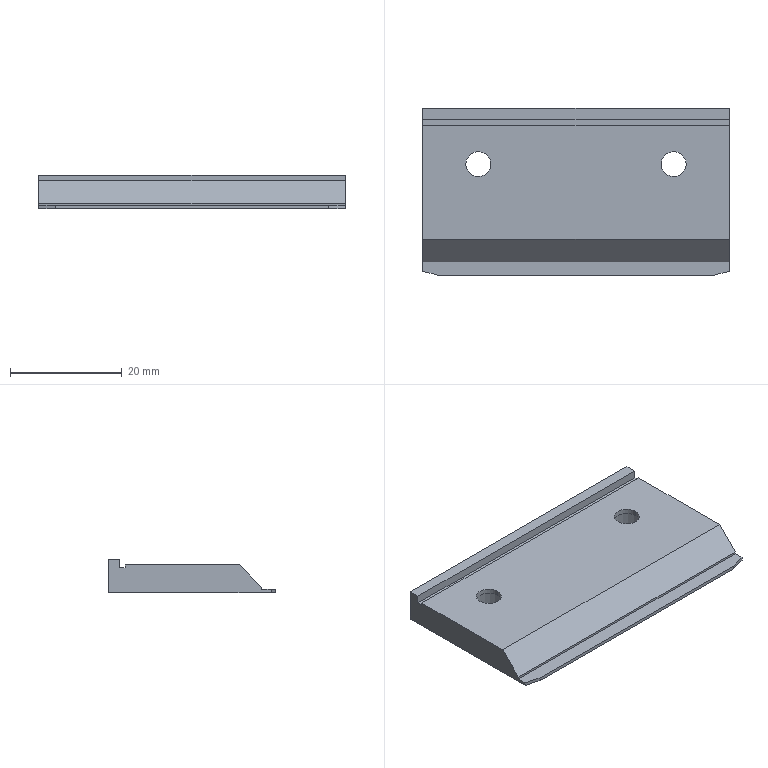Part | STEP file | 11-FG-B03011 | 1 solid | 25 faces | box 55 x 30 x 6 mm | volume 6845 mm3 | plane 17 | cylinder 8 | commonest cylinder face diameters 4.5 x4 8 x4
STEP:
#1=CARTESIAN_POINT('',(14.,20.,-0.9));
#2=VERTEX_POINT('',#1);
#3=CARTESIAN_POINT('',(6.,20.,-0.9));
#4=VERTEX_POINT('',#3);
#5=CARTESIAN_POINT('',(10.,20.,-0.9));
#6=DIRECTION('',(0.,0.,-1.));
#7=DIRECTION('',(-1.,0.,0.));
#8=AXIS2_PLACEMENT_3D('',#5,#6,#7);
#9=CIRCLE('',#8,4.);
#10=EDGE_CURVE('',#2,#4,#9,.T.);
#11=ORIENTED_EDGE('',*,*,#10,.F.);
#12=CARTESIAN_POINT('',(14.,20.,-5.));
#13=VERTEX_POINT('',#12);
#14=CARTESIAN_POINT('',(14.,20.,-5.));
#15=DIRECTION('',(0.,0.,-1.));
#16=VECTOR('',#15,1000.);
#17=LINE('',#14,#16);
#18=EDGE_CURVE('',#2,#13,#17,.T.);
#19=ORIENTED_EDGE('',*,*,#18,.T.);
#20=CARTESIAN_POINT('',(6.,20.,-5.));
#21=VERTEX_POINT('',#20);
#22=CARTESIAN_POINT('',(10.,20.,-5.));
#23=DIRECTION('',(0.,0.,-1.));
#24=DIRECTION('',(-1.,0.,0.));
#25=AXIS2_PLACEMENT_3D('',#22,#23,#24);
#26=CIRCLE('',#25,4.);
#27=EDGE_CURVE('',#13,#21,#26,.T.);
#28=ORIENTED_EDGE('',*,*,#27,.T.);
#29=CARTESIAN_POINT('',(6.,20.,-5.));
#30=DIRECTION('',(0.,0.,-1.));
#31=VECTOR('',#30,1000.);
#32=LINE('',#29,#31);
#33=EDGE_CURVE('',#4,#21,#32,.T.);
#34=ORIENTED_EDGE('',*,*,#33,.F.);
#35=EDGE_LOOP('',(#11,#19,#28,#34));
#36=FACE_OUTER_BOUND('',#35,.T.);
#37=CARTESIAN_POINT('',(10.,20.,-5.));
#38=DIRECTION('',(0.,0.,-1.));
#39=DIRECTION('',(-1.,0.,0.));
#40=AXIS2_PLACEMENT_3D('',#37,#38,#39);
#41=CYLINDRICAL_SURFACE('',#40,4.);
#42=ADVANCED_FACE('',(#36),#41,.F.);
#43=CARTESIAN_POINT('',(12.25,20.,0.));
#44=VERTEX_POINT('',#43);
#45=CARTESIAN_POINT('',(7.75,20.,0.));
#46=VERTEX_POINT('',#45);
#47=CARTESIAN_POINT('',(10.,20.,0.));
#48=DIRECTION('',(0.,0.,-1.));
#49=DIRECTION('',(-1.,0.,0.));
#50=AXIS2_PLACEMENT_3D('',#47,#48,#49);
#51=CIRCLE('',#50,2.25);
#52=EDGE_CURVE('',#44,#46,#51,.T.);
#53=ORIENTED_EDGE('',*,*,#52,.F.);
#54=CARTESIAN_POINT('',(12.25,20.,-0.9));
#55=VERTEX_POINT('',#54);
#56=CARTESIAN_POINT('',(12.25,20.,-5.));
#57=DIRECTION('',(0.,0.,-1.));
#58=VECTOR('',#57,1000.);
#59=LINE('',#56,#58);
#60=EDGE_CURVE('',#44,#55,#59,.T.);
#61=ORIENTED_EDGE('',*,*,#60,.T.);
#62=CARTESIAN_POINT('',(7.75,20.,-0.9));
#63=VERTEX_POINT('',#62);
#64=CARTESIAN_POINT('',(10.,20.,-0.9));
#65=DIRECTION('',(0.,0.,-1.));
#66=DIRECTION('',(-1.,0.,0.));
#67=AXIS2_PLACEMENT_3D('',#64,#65,#66);
#68=CIRCLE('',#67,2.25);
#69=EDGE_CURVE('',#55,#63,#68,.T.);
#70=ORIENTED_EDGE('',*,*,#69,.T.);
#71=CARTESIAN_POINT('',(7.75,20.,-5.));
#72=DIRECTION('',(0.,0.,-1.));
#73=VECTOR('',#72,1000.);
#74=LINE('',#71,#73);
#75=EDGE_CURVE('',#46,#63,#74,.T.);
#76=ORIENTED_EDGE('',*,*,#75,.F.);
#77=EDGE_LOOP('',(#53,#61,#70,#76));
#78=FACE_OUTER_BOUND('',#77,.T.);
#79=CARTESIAN_POINT('',(10.,20.,-5.));
#80=DIRECTION('',(0.,0.,-1.));
#81=DIRECTION('',(-1.,0.,0.));
#82=AXIS2_PLACEMENT_3D('',#79,#80,#81);
#83=CYLINDRICAL_SURFACE('',#82,2.25);
#84=ADVANCED_FACE('',(#78),#83,.F.);
#85=CARTESIAN_POINT('',(49.,20.,-0.9));
#86=VERTEX_POINT('',#85);
#87=CARTESIAN_POINT('',(41.,20.,-0.9));
#88=VERTEX_POINT('',#87);
#89=CARTESIAN_POINT('',(45.,20.,-0.9));
#90=DIRECTION('',(0.,0.,-1.));
#91=DIRECTION('',(-1.,0.,0.));
#92=AXIS2_PLACEMENT_3D('',#89,#90,#91);
#93=CIRCLE('',#92,4.);
#94=EDGE_CURVE('',#86,#88,#93,.T.);
#95=ORIENTED_EDGE('',*,*,#94,.F.);
#96=CARTESIAN_POINT('',(49.,20.,-5.));
#97=VERTEX_POINT('',#96);
#98=CARTESIAN_POINT('',(49.,20.,-5.));
#99=DIRECTION('',(0.,0.,-1.));
#100=VECTOR('',#99,1000.);
#101=LINE('',#98,#100);
#102=EDGE_CURVE('',#86,#97,#101,.T.);
#103=ORIENTED_EDGE('',*,*,#102,.T.);
#104=CARTESIAN_POINT('',(41.,20.,-5.));
#105=VERTEX_POINT('',#104);
#106=CARTESIAN_POINT('',(45.,20.,-5.));
#107=DIRECTION('',(0.,0.,-1.));
#108=DIRECTION('',(-1.,0.,0.));
#109=AXIS2_PLACEMENT_3D('',#106,#107,#108);
#110=CIRCLE('',#109,4.);
#111=EDGE_CURVE('',#97,#105,#110,.T.);
#112=ORIENTED_EDGE('',*,*,#111,.T.);
#113=CARTESIAN_POINT('',(41.,20.,-5.));
#114=DIRECTION('',(0.,0.,-1.));
#115=VECTOR('',#114,1000.);
#116=LINE('',#113,#115);
#117=EDGE_CURVE('',#88,#105,#116,.T.);
#118=ORIENTED_EDGE('',*,*,#117,.F.);
#119=EDGE_LOOP('',(#95,#103,#112,#118));
#120=FACE_OUTER_BOUND('',#119,.T.);
#121=CARTESIAN_POINT('',(45.,20.,-5.));
#122=DIRECTION('',(0.,0.,-1.));
#123=DIRECTION('',(-1.,0.,0.));
#124=AXIS2_PLACEMENT_3D('',#121,#122,#123);
#125=CYLINDRICAL_SURFACE('',#124,4.);
#126=ADVANCED_FACE('',(#120),#125,.F.);
#127=CARTESIAN_POINT('',(47.25,20.,0.));
#128=VERTEX_POINT('',#127);
#129=CARTESIAN_POINT('',(42.75,20.,0.));
#130=VERTEX_POINT('',#129);
#131=CARTESIAN_POINT('',(45.,20.,0.));
#132=DIRECTION('',(0.,0.,-1.));
#133=DIRECTION('',(-1.,0.,0.));
#134=AXIS2_PLACEMENT_3D('',#131,#132,#133);
#135=CIRCLE('',#134,2.25);
#136=EDGE_CURVE('',#128,#130,#135,.T.);
#137=ORIENTED_EDGE('',*,*,#136,.F.);
#138=CARTESIAN_POINT('',(47.25,20.,-0.9));
#139=VERTEX_POINT('',#138);
#140=CARTESIAN_POINT('',(47.25,20.,-5.));
#141=DIRECTION('',(0.,0.,-1.));
#142=VECTOR('',#141,1000.);
#143=LINE('',#140,#142);
#144=EDGE_CURVE('',#128,#139,#143,.T.);
#145=ORIENTED_EDGE('',*,*,#144,.T.);
#146=CARTESIAN_POINT('',(42.75,20.,-0.9));
#147=VERTEX_POINT('',#146);
#148=CARTESIAN_POINT('',(45.,20.,-0.9));
#149=DIRECTION('',(0.,0.,-1.));
#150=DIRECTION('',(-1.,0.,0.));
#151=AXIS2_PLACEMENT_3D('',#148,#149,#150);
#152=CIRCLE('',#151,2.25);
#153=EDGE_CURVE('',#139,#147,#152,.T.);
#154=ORIENTED_EDGE('',*,*,#153,.T.);
#155=CARTESIAN_POINT('',(42.75,20.,-5.));
#156=DIRECTION('',(0.,0.,-1.));
#157=VECTOR('',#156,1000.);
#158=LINE('',#155,#157);
#159=EDGE_CURVE('',#130,#147,#158,.T.);
#160=ORIENTED_EDGE('',*,*,#159,.F.);
#161=EDGE_LOOP('',(#137,#145,#154,#160));
#162=FACE_OUTER_BOUND('',#161,.T.);
#163=CARTESIAN_POINT('',(45.,20.,-5.));
#164=DIRECTION('',(0.,0.,-1.));
#165=DIRECTION('',(-1.,0.,0.));
#166=AXIS2_PLACEMENT_3D('',#163,#164,#165);
#167=CYLINDRICAL_SURFACE('',#166,2.25);
#168=ADVANCED_FACE('',(#162),#167,.F.);
#169=CARTESIAN_POINT('',(10.,20.,0.));
#170=DIRECTION('',(0.,0.,-1.));
#171=DIRECTION('',(-1.,0.,0.));
#172=AXIS2_PLACEMENT_3D('',#169,#170,#171);
#173=CIRCLE('',#172,2.25);
#174=EDGE_CURVE('',#46,#44,#173,.T.);
#175=ORIENTED_EDGE('',*,*,#174,.T.);
#176=ORIENTED_EDGE('',*,*,#52,.T.);
#177=EDGE_LOOP('',(#175,#176));
#178=FACE_BOUND('',#177,.T.);
#179=CARTESIAN_POINT('',(45.,20.,0.));
#180=DIRECTION('',(0.,0.,-1.));
#181=DIRECTION('',(-1.,0.,0.));
#182=AXIS2_PLACEMENT_3D('',#179,#180,#181);
#183=CIRCLE('',#182,2.25);
#184=EDGE_CURVE('',#130,#128,#183,.T.);
#185=ORIENTED_EDGE('',*,*,#184,.T.);
#186=ORIENTED_EDGE('',*,*,#136,.T.);
#187=EDGE_LOOP('',(#185,#186));
#188=FACE_BOUND('',#187,.T.);
#189=CARTESIAN_POINT('',(55.,27.,0.));
#190=VERTEX_POINT('',#189);
#191=CARTESIAN_POINT('',(55.,6.5,0.));
#192=VERTEX_POINT('',#191);
#193=CARTESIAN_POINT('',(55.,30.,0.));
#194=DIRECTION('',(0.,-1.,0.));
#195=VECTOR('',#194,1000.);
#196=LINE('',#193,#195);
#197=EDGE_CURVE('',#190,#192,#196,.T.);
#198=ORIENTED_EDGE('',*,*,#197,.F.);
#199=CARTESIAN_POINT('',(0.,27.,0.));
#200=VERTEX_POINT('',#199);
#201=CARTESIAN_POINT('',(76.,27.,0.));
#202=DIRECTION('',(-1.,0.,0.));
#203=VECTOR('',#202,1000.);
#204=LINE('',#201,#203);
#205=EDGE_CURVE('',#190,#200,#204,.T.);
#206=ORIENTED_EDGE('',*,*,#205,.T.);
#207=CARTESIAN_POINT('',(0.,6.5,0.));
#208=VERTEX_POINT('',#207);
#209=CARTESIAN_POINT('',(0.,30.,0.));
#210=DIRECTION('',(0.,-1.,0.));
#211=VECTOR('',#210,1000.);
#212=LINE('',#209,#211);
#213=EDGE_CURVE('',#200,#208,#212,.T.);
#214=ORIENTED_EDGE('',*,*,#213,.T.);
#215=CARTESIAN_POINT('',(0.,6.5,0.));
#216=DIRECTION('',(1.,0.,0.));
#217=VECTOR('',#216,1000.);
#218=LINE('',#215,#217);
#219=EDGE_CURVE('',#208,#192,#218,.T.);
#220=ORIENTED_EDGE('',*,*,#219,.T.);
#221=EDGE_LOOP('',(#198,#206,#214,#220));
#222=FACE_OUTER_BOUND('',#221,.T.);
#223=CARTESIAN_POINT('',(0.,30.,0.));
#224=DIRECTION('',(0.,0.,-1.));
#225=DIRECTION('',(-1.,0.,0.));
#226=AXIS2_PLACEMENT_3D('',#223,#224,#225);
#227=PLANE('',#226);
#228=ADVANCED_FACE('',(#178,#188,#222),#227,.F.);
#229=ORIENTED_EDGE('',*,*,#213,.F.);
#230=CARTESIAN_POINT('',(0.,27.,-0.5));
#231=VERTEX_POINT('',#230);
#232=CARTESIAN_POINT('',(0.,27.,0.));
#233=DIRECTION('',(0.,0.,1.));
#234=VECTOR('',#233,1000.);
#235=LINE('',#232,#234);
#236=EDGE_CURVE('',#231,#200,#235,.T.);
#237=ORIENTED_EDGE('',*,*,#236,.F.);
#238=CARTESIAN_POINT('',(0.,28.,-0.5));
#239=VERTEX_POINT('',#238);
#240=CARTESIAN_POINT('',(0.,28.,-0.5));
#241=DIRECTION('',(0.,-1.,0.));
#242=VECTOR('',#241,1000.);
#243=LINE('',#240,#242);
#244=EDGE_CURVE('',#239,#231,#243,.T.);
#245=ORIENTED_EDGE('',*,*,#244,.F.);
#246=CARTESIAN_POINT('',(0.,28.,1.));
#247=VERTEX_POINT('',#246);
#248=CARTESIAN_POINT('',(0.,28.,0.));
#249=DIRECTION('',(0.,0.,-1.));
#250=VECTOR('',#249,1000.);
#251=LINE('',#248,#250);
#252=EDGE_CURVE('',#247,#239,#251,.T.);
#253=ORIENTED_EDGE('',*,*,#252,.F.);
#254=CARTESIAN_POINT('',(0.,30.,1.));
#255=VERTEX_POINT('',#254);
#256=CARTESIAN_POINT('',(0.,30.,1.));
#257=DIRECTION('',(0.,-1.,0.));
#258=VECTOR('',#257,1000.);
#259=LINE('',#256,#258);
#260=EDGE_CURVE('',#255,#247,#259,.T.);
#261=ORIENTED_EDGE('',*,*,#260,.F.);
#262=CARTESIAN_POINT('',(0.,30.,-5.));
#263=VERTEX_POINT('',#262);
#264=CARTESIAN_POINT('',(0.,30.,0.));
#265=DIRECTION('',(0.,0.,1.));
#266=VECTOR('',#265,1000.);
#267=LINE('',#264,#266);
#268=EDGE_CURVE('',#263,#255,#267,.T.);
#269=ORIENTED_EDGE('',*,*,#268,.F.);
#270=CARTESIAN_POINT('',(0.,0.8038,-5.));
#271=VERTEX_POINT('',#270);
#272=CARTESIAN_POINT('',(0.,30.,-5.));
#273=DIRECTION('',(0.,-1.,0.));
#274=VECTOR('',#273,1000.);
#275=LINE('',#272,#274);
#276=EDGE_CURVE('',#263,#271,#275,.T.);
#277=ORIENTED_EDGE('',*,*,#276,.T.);
#278=CARTESIAN_POINT('',(0.,0.8038,-4.4));
#279=VERTEX_POINT('',#278);
#280=CARTESIAN_POINT('',(0.,0.8038,0.));
#281=DIRECTION('',(0.,0.,1.));
#282=VECTOR('',#281,1000.);
#283=LINE('',#280,#282);
#284=EDGE_CURVE('',#271,#279,#283,.T.);
#285=ORIENTED_EDGE('',*,*,#284,.T.);
#286=CARTESIAN_POINT('',(0.,2.5,-4.4));
#287=VERTEX_POINT('',#286);
#288=CARTESIAN_POINT('',(0.,0.,-4.4));
#289=DIRECTION('',(0.,1.,0.));
#290=VECTOR('',#289,1000.);
#291=LINE('',#288,#290);
#292=EDGE_CURVE('',#279,#287,#291,.T.);
#293=ORIENTED_EDGE('',*,*,#292,.T.);
#294=CARTESIAN_POINT('',(0.,2.5,-4.));
#295=VERTEX_POINT('',#294);
#296=CARTESIAN_POINT('',(0.,2.5,0.));
#297=DIRECTION('',(0.,0.,1.));
#298=VECTOR('',#297,1000.);
#299=LINE('',#296,#298);
#300=EDGE_CURVE('',#287,#295,#299,.T.);
#301=ORIENTED_EDGE('',*,*,#300,.T.);
#302=CARTESIAN_POINT('',(0.,6.5,0.));
#303=DIRECTION('',(0.,0.7071,0.7071));
#304=VECTOR('',#303,1000.);
#305=LINE('',#302,#304);
#306=EDGE_CURVE('',#295,#208,#305,.T.);
#307=ORIENTED_EDGE('',*,*,#306,.T.);
#308=EDGE_LOOP('',(#229,#237,#245,#253,#261,#269,#277,#285,#293,#301,#307));
#309=FACE_OUTER_BOUND('',#308,.T.);
#310=CARTESIAN_POINT('',(0.,30.,0.));
#311=DIRECTION('',(1.,0.,0.));
#312=DIRECTION('',(0.,0.,-1.));
#313=AXIS2_PLACEMENT_3D('',#310,#311,#312);
#314=PLANE('',#313);
#315=ADVANCED_FACE('',(#309),#314,.F.);
#316=CARTESIAN_POINT('',(55.,28.,-0.5));
#317=VERTEX_POINT('',#316);
#318=CARTESIAN_POINT('',(55.,27.,-0.5));
#319=VERTEX_POINT('',#318);
#320=CARTESIAN_POINT('',(55.,30.,-0.5));
#321=DIRECTION('',(0.,-1.,0.));
#322=VECTOR('',#321,1000.);
#323=LINE('',#320,#322);
#324=EDGE_CURVE('',#317,#319,#323,.T.);
#325=ORIENTED_EDGE('',*,*,#324,.T.);
#326=CARTESIAN_POINT('',(55.,27.,0.));
#327=DIRECTION('',(0.,0.,1.));
#328=VECTOR('',#327,1000.);
#329=LINE('',#326,#328);
#330=EDGE_CURVE('',#319,#190,#329,.T.);
#331=ORIENTED_EDGE('',*,*,#330,.T.);
#332=ORIENTED_EDGE('',*,*,#197,.T.);
#333=CARTESIAN_POINT('',(55.,2.5,-4.));
#334=VERTEX_POINT('',#333);
#335=CARTESIAN_POINT('',(55.,6.5,0.));
#336=DIRECTION('',(0.,-0.7071,-0.7071));
#337=VECTOR('',#336,1000.);
#338=LINE('',#335,#337);
#339=EDGE_CURVE('',#192,#334,#338,.T.);
#340=ORIENTED_EDGE('',*,*,#339,.T.);
#341=CARTESIAN_POINT('',(55.,2.5,-4.4));
#342=VERTEX_POINT('',#341);
#343=CARTESIAN_POINT('',(55.,2.5,0.));
#344=DIRECTION('',(0.,0.,1.));
#345=VECTOR('',#344,1000.);
#346=LINE('',#343,#345);
#347=EDGE_CURVE('',#342,#334,#346,.T.);
#348=ORIENTED_EDGE('',*,*,#347,.F.);
#349=CARTESIAN_POINT('',(55.,0.8038,-4.4));
#350=VERTEX_POINT('',#349);
#351=CARTESIAN_POINT('',(55.,0.,-4.4));
#352=DIRECTION('',(0.,1.,0.));
#353=VECTOR('',#352,1000.);
#354=LINE('',#351,#353);
#355=EDGE_CURVE('',#350,#342,#354,.T.);
#356=ORIENTED_EDGE('',*,*,#355,.F.);
#357=CARTESIAN_POINT('',(55.,0.8038,-5.));
#358=VERTEX_POINT('',#357);
#359=CARTESIAN_POINT('',(55.,0.8038,-5.));
#360=DIRECTION('',(0.,0.,-1.));
#361=VECTOR('',#360,1000.);
#362=LINE('',#359,#361);
#363=EDGE_CURVE('',#350,#358,#362,.T.);
#364=ORIENTED_EDGE('',*,*,#363,.T.);
#365=CARTESIAN_POINT('',(55.,30.,-5.));
#366=VERTEX_POINT('',#365);
#367=CARTESIAN_POINT('',(55.,30.,-5.));
#368=DIRECTION('',(0.,-1.,0.));
#369=VECTOR('',#368,1000.);
#370=LINE('',#367,#369);
#371=EDGE_CURVE('',#366,#358,#370,.T.);
#372=ORIENTED_EDGE('',*,*,#371,.F.);
#373=CARTESIAN_POINT('',(55.,30.,1.));
#374=VERTEX_POINT('',#373);
#375=CARTESIAN_POINT('',(55.,30.,0.));
#376=DIRECTION('',(0.,0.,-1.));
#377=VECTOR('',#376,1000.);
#378=LINE('',#375,#377);
#379=EDGE_CURVE('',#374,#366,#378,.T.);
#380=ORIENTED_EDGE('',*,*,#379,.F.);
#381=CARTESIAN_POINT('',(55.,28.,1.));
#382=VERTEX_POINT('',#381);
#383=CARTESIAN_POINT('',(55.,30.,1.));
#384=DIRECTION('',(0.,-1.,0.));
#385=VECTOR('',#384,1000.);
#386=LINE('',#383,#385);
#387=EDGE_CURVE('',#374,#382,#386,.T.);
#388=ORIENTED_EDGE('',*,*,#387,.T.);
#389=CARTESIAN_POINT('',(55.,28.,0.));
#390=DIRECTION('',(0.,0.,-1.));
#391=VECTOR('',#390,1000.);
#392=LINE('',#389,#391);
#393=EDGE_CURVE('',#382,#317,#392,.T.);
#394=ORIENTED_EDGE('',*,*,#393,.T.);
#395=EDGE_LOOP('',(#325,#331,#332,#340,#348,#356,#364,#372,#380,#388,#394));
#396=FACE_OUTER_BOUND('',#395,.T.);
#397=CARTESIAN_POINT('',(55.,30.,0.));
#398=DIRECTION('',(-1.,0.,0.));
#399=DIRECTION('',(0.,0.,1.));
#400=AXIS2_PLACEMENT_3D('',#397,#398,#399);
#401=PLANE('',#400);
#402=ADVANCED_FACE('',(#396),#401,.F.);
#403=CARTESIAN_POINT('',(10.,20.,-5.));
#404=DIRECTION('',(0.,0.,-1.));
#405=DIRECTION('',(-1.,0.,0.));
#406=AXIS2_PLACEMENT_3D('',#403,#404,#405);
#407=CIRCLE('',#406,4.);
#408=EDGE_CURVE('',#21,#13,#407,.T.);
#409=ORIENTED_EDGE('',*,*,#408,.F.);
#410=ORIENTED_EDGE('',*,*,#27,.F.);
#411=EDGE_LOOP('',(#409,#410));
#412=FACE_BOUND('',#411,.T.);
#413=CARTESIAN_POINT('',(45.,20.,-5.));
#414=DIRECTION('',(0.,0.,-1.));
#415=DIRECTION('',(-1.,0.,0.));
#416=AXIS2_PLACEMENT_3D('',#413,#414,#415);
#417=CIRCLE('',#416,4.);
#418=EDGE_CURVE('',#105,#97,#417,.T.);
#419=ORIENTED_EDGE('',*,*,#418,.F.);
#420=ORIENTED_EDGE('',*,*,#111,.F.);
#421=EDGE_LOOP('',(#419,#420));
#422=FACE_BOUND('',#421,.T.);
#423=ORIENTED_EDGE('',*,*,#371,.T.);
#424=CARTESIAN_POINT('',(52.,0.,-5.));
#425=VERTEX_POINT('',#424);
#426=CARTESIAN_POINT('',(55.,0.8038,-5.));
#427=DIRECTION('',(-0.9659,-0.2588,0.));
#428=VECTOR('',#427,1000.);
#429=LINE('',#426,#428);
#430=EDGE_CURVE('',#358,#425,#429,.T.);
#431=ORIENTED_EDGE('',*,*,#430,.T.);
#432=CARTESIAN_POINT('',(3.,0.,-5.));
#433=VERTEX_POINT('',#432);
#434=CARTESIAN_POINT('',(0.,0.,-5.));
#435=DIRECTION('',(-1.,0.,0.));
#436=VECTOR('',#435,1000.);
#437=LINE('',#434,#436);
#438=EDGE_CURVE('',#425,#433,#437,.T.);
#439=ORIENTED_EDGE('',*,*,#438,.T.);
#440=CARTESIAN_POINT('',(0.,0.8038,-5.));
#441=DIRECTION('',(-0.9659,0.2588,0.));
#442=VECTOR('',#441,1000.);
#443=LINE('',#440,#442);
#444=EDGE_CURVE('',#433,#271,#443,.T.);
#445=ORIENTED_EDGE('',*,*,#444,.T.);
#446=ORIENTED_EDGE('',*,*,#276,.F.);
#447=CARTESIAN_POINT('',(0.,30.,-5.));
#448=DIRECTION('',(-1.,0.,0.));
#449=VECTOR('',#448,1000.);
#450=LINE('',#447,#449);
#451=EDGE_CURVE('',#366,#263,#450,.T.);
#452=ORIENTED_EDGE('',*,*,#451,.F.);
#453=EDGE_LOOP('',(#423,#431,#439,#445,#446,#452));
#454=FACE_OUTER_BOUND('',#453,.T.);
#455=CARTESIAN_POINT('',(0.,30.,-5.));
#456=DIRECTION('',(0.,0.,1.));
#457=DIRECTION('',(1.,0.,0.));
#458=AXIS2_PLACEMENT_3D('',#455,#456,#457);
#459=PLANE('',#458);
#460=ADVANCED_FACE('',(#412,#422,#454),#459,.F.);
#461=ORIENTED_EDGE('',*,*,#268,.T.);
#462=CARTESIAN_POINT('',(0.,30.,1.));
#463=DIRECTION('',(1.,0.,0.));
#464=VECTOR('',#463,1000.);
#465=LINE('',#462,#464);
#466=EDGE_CURVE('',#255,#374,#465,.T.);
#467=ORIENTED_EDGE('',*,*,#466,.T.);
#468=ORIENTED_EDGE('',*,*,#379,.T.);
#469=ORIENTED_EDGE('',*,*,#451,.T.);
#470=EDGE_LOOP('',(#461,#467,#468,#469));
#471=FACE_OUTER_BOUND('',#470,.T.);
#472=CARTESIAN_POINT('',(0.,30.,-5.));
#473=DIRECTION('',(0.,-1.,0.));
#474=DIRECTION('',(0.,0.,-1.));
#475=AXIS2_PLACEMENT_3D('',#472,#473,#474);
#476=PLANE('',#475);
#477=ADVANCED_FACE('',(#471),#476,.F.);
#478=CARTESIAN_POINT('',(3.,0.,-4.4));
#479=VERTEX_POINT('',#478);
#480=CARTESIAN_POINT('',(52.,0.,-4.4));
#481=VERTEX_POINT('',#480);
#482=CARTESIAN_POINT('',(0.,0.,-4.4));
#483=DIRECTION('',(1.,0.,0.));
#484=VECTOR('',#483,1000.);
#485=LINE('',#482,#484);
#486=EDGE_CURVE('',#479,#481,#485,.T.);
#487=ORIENTED_EDGE('',*,*,#486,.F.);
#488=CARTESIAN_POINT('',(3.,0.,-5.));
#489=DIRECTION('',(0.,0.,-1.));
#490=VECTOR('',#489,1000.);
#491=LINE('',#488,#490);
#492=EDGE_CURVE('',#479,#433,#491,.T.);
#493=ORIENTED_EDGE('',*,*,#492,.T.);
#494=ORIENTED_EDGE('',*,*,#438,.F.);
#495=CARTESIAN_POINT('',(52.,0.,0.));
#496=DIRECTION('',(0.,0.,1.));
#497=VECTOR('',#496,1000.);
#498=LINE('',#495,#497);
#499=EDGE_CURVE('',#425,#481,#498,.T.);
#500=ORIENTED_EDGE('',*,*,#499,.T.);
#501=EDGE_LOOP('',(#487,#493,#494,#500));
#502=FACE_OUTER_BOUND('',#501,.T.);
#503=CARTESIAN_POINT('',(0.,0.,-5.));
#504=DIRECTION('',(0.,-1.,0.));
#505=DIRECTION('',(0.,0.,-1.));
#506=AXIS2_PLACEMENT_3D('',#503,#504,#505);
#507=PLANE('',#506);
#508=ADVANCED_FACE('',(#502),#507,.T.);
#509=CARTESIAN_POINT('',(55.,0.8038,-4.4));
#510=DIRECTION('',(0.9659,0.2588,0.));
#511=VECTOR('',#510,1000.);
#512=LINE('',#509,#511);
#513=EDGE_CURVE('',#481,#350,#512,.T.);
#514=ORIENTED_EDGE('',*,*,#513,.F.);
#515=ORIENTED_EDGE('',*,*,#499,.F.);
#516=ORIENTED_EDGE('',*,*,#430,.F.);
#517=ORIENTED_EDGE('',*,*,#363,.F.);
#518=EDGE_LOOP('',(#514,#515,#516,#517));
#519=FACE_OUTER_BOUND('',#518,.T.);
#520=CARTESIAN_POINT('',(55.,0.8038,0.));
#521=DIRECTION('',(0.2588,-0.9659,0.));
#522=DIRECTION('',(0.9659,0.2588,0.));
#523=AXIS2_PLACEMENT_3D('',#520,#521,#522);
#524=PLANE('',#523);
#525=ADVANCED_FACE('',(#519),#524,.T.);
#526=CARTESIAN_POINT('',(0.,0.8038,-4.4));
#527=DIRECTION('',(0.9659,-0.2588,0.));
#528=VECTOR('',#527,1000.);
#529=LINE('',#526,#528);
#530=EDGE_CURVE('',#279,#479,#529,.T.);
#531=ORIENTED_EDGE('',*,*,#530,.F.);
#532=ORIENTED_EDGE('',*,*,#284,.F.);
#533=ORIENTED_EDGE('',*,*,#444,.F.);
#534=ORIENTED_EDGE('',*,*,#492,.F.);
#535=EDGE_LOOP('',(#531,#532,#533,#534));
#536=FACE_OUTER_BOUND('',#535,.T.);
#537=CARTESIAN_POINT('',(0.,0.8038,0.));
#538=DIRECTION('',(-0.2588,-0.9659,0.));
#539=DIRECTION('',(0.9659,-0.2588,0.));
#540=AXIS2_PLACEMENT_3D('',#537,#538,#539);
#541=PLANE('',#540);
#542=ADVANCED_FACE('',(#536),#541,.T.);
#543=ORIENTED_EDGE('',*,*,#347,.T.);
#544=CARTESIAN_POINT('',(0.,2.5,-4.));
#545=DIRECTION('',(-1.,0.,0.));
#546=VECTOR('',#545,1000.);
#547=LINE('',#544,#546);
#548=EDGE_CURVE('',#334,#295,#547,.T.);
#549=ORIENTED_EDGE('',*,*,#548,.T.);
#550=ORIENTED_EDGE('',*,*,#300,.F.);
#551=CARTESIAN_POINT('',(0.,2.5,-4.4));
#552=DIRECTION('',(1.,0.,0.));
#553=VECTOR('',#552,1000.);
#554=LINE('',#551,#553);
#555=EDGE_CURVE('',#287,#342,#554,.T.);
#556=ORIENTED_EDGE('',*,*,#555,.T.);
#557=EDGE_LOOP('',(#543,#549,#550,#556));
#558=FACE_OUTER_BOUND('',#557,.T.);
#559=CARTESIAN_POINT('',(0.,2.5,0.));
#560=DIRECTION('',(0.,1.,0.));
#561=DIRECTION('',(0.,0.,1.));
#562=AXIS2_PLACEMENT_3D('',#559,#560,#561);
#563=PLANE('',#562);
#564=ADVANCED_FACE('',(#558),#563,.F.);
#565=ORIENTED_EDGE('',*,*,#513,.T.);
#566=ORIENTED_EDGE('',*,*,#355,.T.);
#567=ORIENTED_EDGE('',*,*,#555,.F.);
#568=ORIENTED_EDGE('',*,*,#292,.F.);
#569=ORIENTED_EDGE('',*,*,#530,.T.);
#570=ORIENTED_EDGE('',*,*,#486,.T.);
#571=EDGE_LOOP('',(#565,#566,#567,#568,#569,#570));
#572=FACE_OUTER_BOUND('',#571,.T.);
#573=CARTESIAN_POINT('',(0.,0.,-4.4));
#574=DIRECTION('',(0.,0.,-1.));
#575=DIRECTION('',(-1.,0.,0.));
#576=AXIS2_PLACEMENT_3D('',#573,#574,#575);
#577=PLANE('',#576);
#578=ADVANCED_FACE('',(#572),#577,.F.);
#579=ORIENTED_EDGE('',*,*,#306,.F.);
#580=ORIENTED_EDGE('',*,*,#548,.F.);
#581=ORIENTED_EDGE('',*,*,#339,.F.);
#582=ORIENTED_EDGE('',*,*,#219,.F.);
#583=EDGE_LOOP('',(#579,#580,#581,#582));
#584=FACE_OUTER_BOUND('',#583,.T.);
#585=CARTESIAN_POINT('',(0.,6.5,0.));
#586=DIRECTION('',(0.,0.7071,-0.7071));
#587=DIRECTION('',(0.,0.7071,0.7071));
#588=AXIS2_PLACEMENT_3D('',#585,#586,#587);
#589=PLANE('',#588);
#590=ADVANCED_FACE('',(#584),#589,.F.);
#591=ORIENTED_EDGE('',*,*,#393,.F.);
#592=CARTESIAN_POINT('',(0.,28.,1.));
#593=DIRECTION('',(1.,0.,0.));
#594=VECTOR('',#593,1000.);
#595=LINE('',#592,#594);
#596=EDGE_CURVE('',#247,#382,#595,.T.);
#597=ORIENTED_EDGE('',*,*,#596,.F.);
#598=ORIENTED_EDGE('',*,*,#252,.T.);
#599=CARTESIAN_POINT('',(76.,28.,-0.5));
#600=DIRECTION('',(-1.,0.,0.));
#601=VECTOR('',#600,1000.);
#602=LINE('',#599,#601);
#603=EDGE_CURVE('',#317,#239,#602,.T.);
#604=ORIENTED_EDGE('',*,*,#603,.F.);
#605=EDGE_LOOP('',(#591,#597,#598,#604));
#606=FACE_OUTER_BOUND('',#605,.T.);
#607=CARTESIAN_POINT('',(0.,28.,0.));
#608=DIRECTION('',(0.,-1.,0.));
#609=DIRECTION('',(0.,0.,-1.));
#610=AXIS2_PLACEMENT_3D('',#607,#608,#609);
#611=PLANE('',#610);
#612=ADVANCED_FACE('',(#606),#611,.T.);
#613=ORIENTED_EDGE('',*,*,#387,.F.);
#614=ORIENTED_EDGE('',*,*,#466,.F.);
#615=ORIENTED_EDGE('',*,*,#260,.T.);
#616=ORIENTED_EDGE('',*,*,#596,.T.);
#617=EDGE_LOOP('',(#613,#614,#615,#616));
#618=FACE_OUTER_BOUND('',#617,.T.);
#619=CARTESIAN_POINT('',(0.,30.,1.));
#620=DIRECTION('',(0.,0.,1.));
#621=DIRECTION('',(1.,0.,0.));
#622=AXIS2_PLACEMENT_3D('',#619,#620,#621);
#623=PLANE('',#622);
#624=ADVANCED_FACE('',(#618),#623,.T.);
#625=ORIENTED_EDGE('',*,*,#144,.F.);
#626=ORIENTED_EDGE('',*,*,#184,.F.);
#627=ORIENTED_EDGE('',*,*,#159,.T.);
#628=CARTESIAN_POINT('',(45.,20.,-0.9));
#629=DIRECTION('',(0.,0.,-1.));
#630=DIRECTION('',(-1.,0.,0.));
#631=AXIS2_PLACEMENT_3D('',#628,#629,#630);
#632=CIRCLE('',#631,2.25);
#633=EDGE_CURVE('',#147,#139,#632,.T.);
#634=ORIENTED_EDGE('',*,*,#633,.T.);
#635=EDGE_LOOP('',(#625,#626,#627,#634));
#636=FACE_OUTER_BOUND('',#635,.T.);
#637=CARTESIAN_POINT('',(45.,20.,-5.));
#638=DIRECTION('',(0.,0.,-1.));
#639=DIRECTION('',(-1.,0.,0.));
#640=AXIS2_PLACEMENT_3D('',#637,#638,#639);
#641=CYLINDRICAL_SURFACE('',#640,2.25);
#642=ADVANCED_FACE('',(#636),#641,.F.);
#643=ORIENTED_EDGE('',*,*,#102,.F.);
#644=CARTESIAN_POINT('',(45.,20.,-0.9));
#645=DIRECTION('',(0.,0.,-1.));
#646=DIRECTION('',(-1.,0.,0.));
#647=AXIS2_PLACEMENT_3D('',#644,#645,#646);
#648=CIRCLE('',#647,4.);
#649=EDGE_CURVE('',#88,#86,#648,.T.);
#650=ORIENTED_EDGE('',*,*,#649,.F.);
#651=ORIENTED_EDGE('',*,*,#117,.T.);
#652=ORIENTED_EDGE('',*,*,#418,.T.);
#653=EDGE_LOOP('',(#643,#650,#651,#652));
#654=FACE_OUTER_BOUND('',#653,.T.);
#655=CARTESIAN_POINT('',(45.,20.,-5.));
#656=DIRECTION('',(0.,0.,-1.));
#657=DIRECTION('',(-1.,0.,0.));
#658=AXIS2_PLACEMENT_3D('',#655,#656,#657);
#659=CYLINDRICAL_SURFACE('',#658,4.);
#660=ADVANCED_FACE('',(#654),#659,.F.);
#661=ORIENTED_EDGE('',*,*,#60,.F.);
#662=ORIENTED_EDGE('',*,*,#174,.F.);
#663=ORIENTED_EDGE('',*,*,#75,.T.);
#664=CARTESIAN_POINT('',(10.,20.,-0.9));
#665=DIRECTION('',(0.,0.,-1.));
#666=DIRECTION('',(-1.,0.,0.));
#667=AXIS2_PLACEMENT_3D('',#664,#665,#666);
#668=CIRCLE('',#667,2.25);
#669=EDGE_CURVE('',#63,#55,#668,.T.);
#670=ORIENTED_EDGE('',*,*,#669,.T.);
#671=EDGE_LOOP('',(#661,#662,#663,#670));
#672=FACE_OUTER_BOUND('',#671,.T.);
#673=CARTESIAN_POINT('',(10.,20.,-5.));
#674=DIRECTION('',(0.,0.,-1.));
#675=DIRECTION('',(-1.,0.,0.));
#676=AXIS2_PLACEMENT_3D('',#673,#674,#675);
#677=CYLINDRICAL_SURFACE('',#676,2.25);
#678=ADVANCED_FACE('',(#672),#677,.F.);
#679=ORIENTED_EDGE('',*,*,#18,.F.);
#680=CARTESIAN_POINT('',(10.,20.,-0.9));
#681=DIRECTION('',(0.,0.,-1.));
#682=DIRECTION('',(-1.,0.,0.));
#683=AXIS2_PLACEMENT_3D('',#680,#681,#682);
#684=CIRCLE('',#683,4.);
#685=EDGE_CURVE('',#4,#2,#684,.T.);
#686=ORIENTED_EDGE('',*,*,#685,.F.);
#687=ORIENTED_EDGE('',*,*,#33,.T.);
#688=ORIENTED_EDGE('',*,*,#408,.T.);
#689=EDGE_LOOP('',(#679,#686,#687,#688));
#690=FACE_OUTER_BOUND('',#689,.T.);
#691=CARTESIAN_POINT('',(10.,20.,-5.));
#692=DIRECTION('',(0.,0.,-1.));
#693=DIRECTION('',(-1.,0.,0.));
#694=AXIS2_PLACEMENT_3D('',#691,#692,#693);
#695=CYLINDRICAL_SURFACE('',#694,4.);
#696=ADVANCED_FACE('',(#690),#695,.F.);
#697=ORIENTED_EDGE('',*,*,#649,.T.);
#698=ORIENTED_EDGE('',*,*,#94,.T.);
#699=EDGE_LOOP('',(#697,#698));
#700=FACE_OUTER_BOUND('',#699,.T.);
#701=ORIENTED_EDGE('',*,*,#633,.F.);
#702=ORIENTED_EDGE('',*,*,#153,.F.);
#703=EDGE_LOOP('',(#701,#702));
#704=FACE_BOUND('',#703,.T.);
#705=CARTESIAN_POINT('',(45.,20.,-0.9));
#706=DIRECTION('',(0.,0.,-1.));
#707=DIRECTION('',(-1.,0.,0.));
#708=AXIS2_PLACEMENT_3D('',#705,#706,#707);
#709=PLANE('',#708);
#710=ADVANCED_FACE('',(#700,#704),#709,.T.);
#711=ORIENTED_EDGE('',*,*,#685,.T.);
#712=ORIENTED_EDGE('',*,*,#10,.T.);
#713=EDGE_LOOP('',(#711,#712));
#714=FACE_OUTER_BOUND('',#713,.T.);
#715=ORIENTED_EDGE('',*,*,#669,.F.);
#716=ORIENTED_EDGE('',*,*,#69,.F.);
#717=EDGE_LOOP('',(#715,#716));
#718=FACE_BOUND('',#717,.T.);
#719=CARTESIAN_POINT('',(10.,20.,-0.9));
#720=DIRECTION('',(0.,0.,-1.));
#721=DIRECTION('',(-1.,0.,0.));
#722=AXIS2_PLACEMENT_3D('',#719,#720,#721);
#723=PLANE('',#722);
#724=ADVANCED_FACE('',(#714,#718),#723,.T.);
#725=CARTESIAN_POINT('',(76.,27.,-0.5));
#726=DIRECTION('',(-1.,0.,0.));
#727=VECTOR('',#726,1000.);
#728=LINE('',#725,#727);
#729=EDGE_CURVE('',#319,#231,#728,.T.);
#730=ORIENTED_EDGE('',*,*,#729,.T.);
#731=ORIENTED_EDGE('',*,*,#236,.T.);
#732=ORIENTED_EDGE('',*,*,#205,.F.);
#733=ORIENTED_EDGE('',*,*,#330,.F.);
#734=EDGE_LOOP('',(#730,#731,#732,#733));
#735=FACE_OUTER_BOUND('',#734,.T.);
#736=CARTESIAN_POINT('',(76.,27.,0.));
#737=DIRECTION('',(0.,-1.,0.));
#738=DIRECTION('',(0.,0.,-1.));
#739=AXIS2_PLACEMENT_3D('',#736,#737,#738);
#740=PLANE('',#739);
#741=ADVANCED_FACE('',(#735),#740,.F.);
#742=ORIENTED_EDGE('',*,*,#603,.T.);
#743=ORIENTED_EDGE('',*,*,#244,.T.);
#744=ORIENTED_EDGE('',*,*,#729,.F.);
#745=ORIENTED_EDGE('',*,*,#324,.F.);
#746=EDGE_LOOP('',(#742,#743,#744,#745));
#747=FACE_OUTER_BOUND('',#746,.T.);
#748=CARTESIAN_POINT('',(76.,28.,-0.5));
#749=DIRECTION('',(0.,0.,-1.));
#750=DIRECTION('',(-1.,0.,0.));
#751=AXIS2_PLACEMENT_3D('',#748,#749,#750);
#752=PLANE('',#751);
#753=ADVANCED_FACE('',(#747),#752,.F.);
#754=CLOSED_SHELL('',(#42,#84,#126,#168,#228,#315,#402,#460,#477,#508,#525,#542,#564,#578,#590,#612,#624,#642,#660,#678,#696,#710,#724,#741,#753));
#755=MANIFOLD_SOLID_BREP('',#754);
#756=CARTESIAN_POINT('',(0.,0.,0.));
#757=DIRECTION('',(0.,0.,1.));
#758=DIRECTION('',(1.,0.,0.));
#759=AXIS2_PLACEMENT_3D('',#756,#757,#758);
#760=(LENGTH_UNIT()NAMED_UNIT(*)SI_UNIT(.MILLI.,.METRE.));
#761=UNCERTAINTY_MEASURE_WITH_UNIT(LENGTH_MEASURE(0.00001),#760,'','');
#762=(NAMED_UNIT(*)PLANE_ANGLE_UNIT()SI_UNIT($,.RADIAN.));
#763=(NAMED_UNIT(*)SI_UNIT($,.STERADIAN.)SOLID_ANGLE_UNIT());
#764=(GEOMETRIC_REPRESENTATION_CONTEXT(3)GLOBAL_UNCERTAINTY_ASSIGNED_CONTEXT((#761))GLOBAL_UNIT_ASSIGNED_CONTEXT((#760,#762,#763))REPRESENTATION_CONTEXT('',''));
#765=ADVANCED_BREP_SHAPE_REPRESENTATION('',(#755,#759),#764);